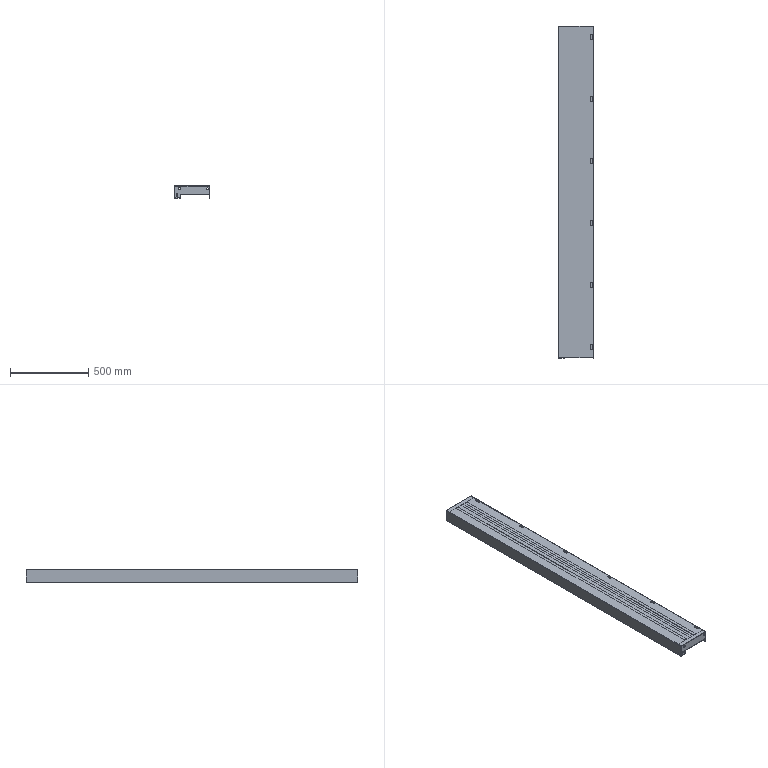Part | SolidWorks | features InContextFeatHolder 1, MirrorCompFeat 1, ReferencePattern 1 | 7 solids | 494 faces | box 226 x 2116 x 80 mm | volume 2102242 mm3 | plane 282 | cylinder 212 | commonest cylinder face diameters 6 x116 6.2 x28 9 x18 11 x10 3.4 x9 10 x6